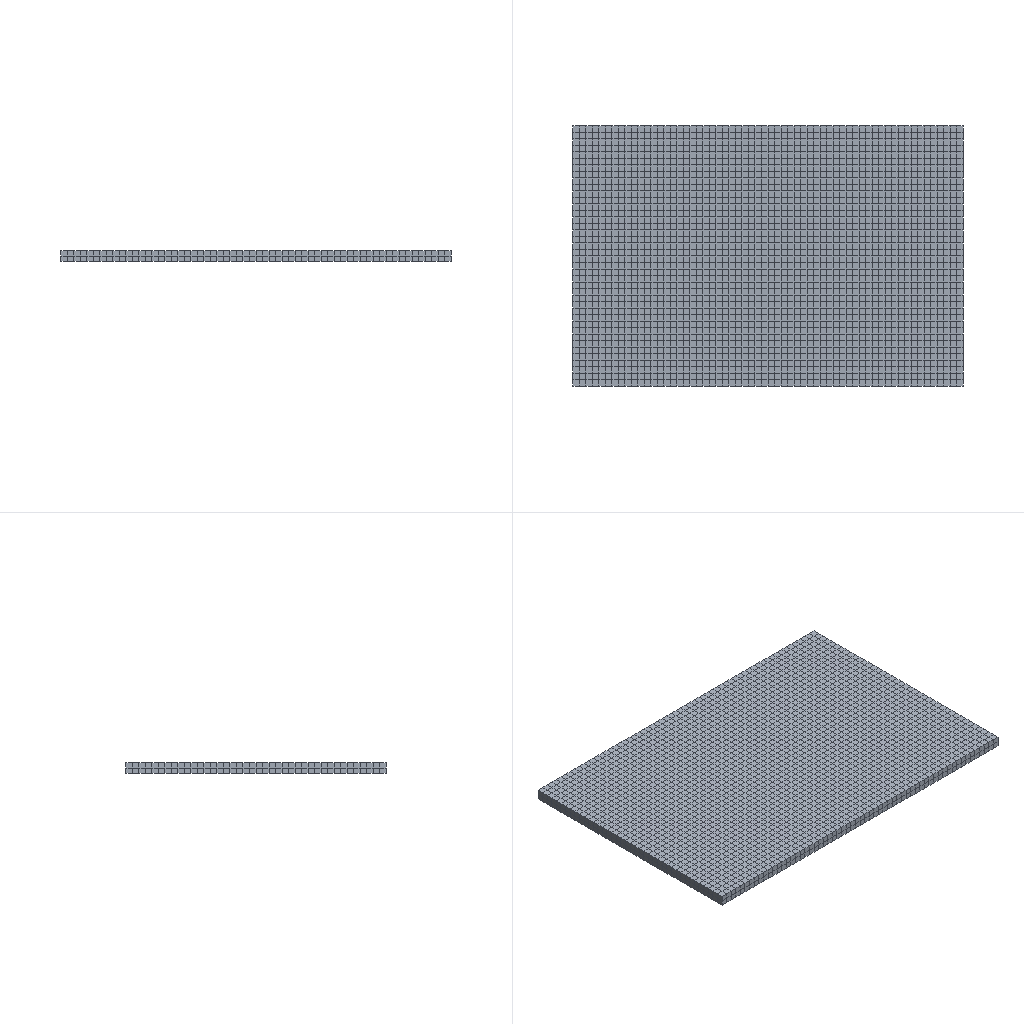Simulation study | abaqus
Set-up summary:
category,name,step,type,value,unit,region
solver,abaqus
solver,version,,,Abaqus/Standard 3DEXPERIENCE R2017x
units,not stated in the deck,,not stated
analysis,deck,,thermal,thermal
load_step,Step-1,Step-1,thermal
load_step,requested,,,1
mesh,nodes,,,7503
mesh,elements,,,4800
element_type,DC3D8,,solid,4800
load,load commands in deck,,count,3
bc,support commands in deck,,count,2
material,MATERIAL-1,,in results
check,setup vs results,,match,"per instance, exact: element labels, types and connectivity; labels of the nodes the elements use; coordinates of those nodes at SINGLE_PRECISION in 1 of 1 instance(s)"
Abaqus input file, long lists of numbers shortened:
*Heading
** Job name: Job-1 Model name: Model-1
** Generated by: Abaqus/CAE 2017
*Preprint, echo=NO, model=NO, history=NO, contact=NO
**
** PARTS
**
*Part, name=Part-1
*Node
      1,           0.,          -6.,           0.
      2,           0.,          -6.,          0.5
** (7501 more lines like these left out)
*Element, type=DC3D8
   1,  210, 2805, 5262,  563,    1,   13,  525,   52
   2, 2805,  270, 1684, 5262,   13,    2,   14,  525
** (4798 more lines like these left out)
*Nset, nset=Set-1, generate
    1,  7503,     1
*Elset, elset=Set-1, generate
    1,  4800,     1
** Section: Section-1
*Solid Section, elset=Set-1, material=Material-1
,
*End Part
**
**
** ASSEMBLY
**
*Assembly, name=Assembly
**
*Instance, name=Part-1-1, part=Part-1
          0.,           6.,           0.
*End Instance
**
*Nset, nset=Set-1, instance=Part-1-1, generate
    1,  7503,     1
*Elset, elset=Set-1, instance=Part-1-1, generate
    1,  4800,     1
*Nset, nset=Set-2, instance=Part-1-1, generate
    1,  7503,     1
*Elset, elset=Set-2, instance=Part-1-1, generate
    1,  4800,     1
*Elset, elset=_Surf-1_S6, internal, instance=Part-1-1, generate
    1,  4799,     2
*Elset, elset=_Surf-1_S1, internal, instance=Part-1-1
 2361, 2362, 2363, 2364, 2365, 2366, 2367, 2368, 2369, 2370, 2371, 2372, 2373, 2374, 2375, 2376
 2377, 2378, 2379, 2380, 2381, 2382, 2383, 2384, 2385, 2386, 2387, 2388, 2389, 2390, 2391, 2392
** (3 more lines like these left out)
*Elset, elset=_Surf-1_S2, internal, instance=Part-1-1
    1,    2,    3,    4,    5,    6,    7,    8,    9,   10,   11,   12,   13,   14,   15,   16
   17,   18,   19,   20,   21,   22,   23,   24,   25,   26,   27,   28,   29,   30,   31,   32
** (3 more lines like these left out)
*Elset, elset=_Surf-1_S5, internal, instance=Part-1-1
   39,   40,   79,   80,  119,  120,  159,  160,  199,  200,  239,  240,  279,  280,  319,  320
  359,  360,  399,  400,  439,  440,  479,  480,  519,  520,  559,  560,  599,  600,  639,  640
** (13 more lines like these left out)
*Elset, elset=_Surf-1_S4, internal, instance=Part-1-1, generate
    2,  4800,     2
*Surface, type=ELEMENT, name=Surf-1
_Surf-1_S6, S6
_Surf-1_S1, S1
_Surf-1_S2, S2
_Surf-1_S4, S4
_Surf-1_S5, S5
*Elset, elset=_Surf-2_S6, internal, instance=Part-1-1, generate
    1,  4799,     2
*Elset, elset=_Surf-2_S1, internal, instance=Part-1-1
 2361, 2362, 2363, 2364, 2365, 2366, 2367, 2368, 2369, 2370, 2371, 2372, 2373, 2374, 2375, 2376
 2377, 2378, 2379, 2380, 2381, 2382, 2383, 2384, 2385, 2386, 2387, 2388, 2389, 2390, 2391, 2392
** (3 more lines like these left out)
*Elset, elset=_Surf-2_S2, internal, instance=Part-1-1
    1,    2,    3,    4,    5,    6,    7,    8,    9,   10,   11,   12,   13,   14,   15,   16
   17,   18,   19,   20,   21,   22,   23,   24,   25,   26,   27,   28,   29,   30,   31,   32
** (3 more lines like these left out)
*Elset, elset=_Surf-2_S5, internal, instance=Part-1-1
   39,   40,   79,   80,  119,  120,  159,  160,  199,  200,  239,  240,  279,  280,  319,  320
  359,  360,  399,  400,  439,  440,  479,  480,  519,  520,  559,  560,  599,  600,  639,  640
** (13 more lines like these left out)
*Elset, elset=_Surf-2_S4, internal, instance=Part-1-1, generate
    2,  4800,     2
*Surface, type=ELEMENT, name=Surf-2
_Surf-2_S6, S6
_Surf-2_S1, S1
_Surf-2_S2, S2
_Surf-2_S4, S4
_Surf-2_S5, S5
*End Assembly
**
** MATERIALS
**
*Material, name=Material-1
*Conductivity
225.,
*Density
 2.7e-09,
*Elastic
320000., 0.25
*Expansion
 6.7e-06,
*Specific Heat
 7.8e+08,
**
** PHYSICAL CONSTANTS
**
*Physical Constants, absolute zero=-273., stefan boltzmann=5.67e-08
**
** PREDEFINED FIELDS
**
** Name: Predefined Field-1   Type: Temperature
*Initial Conditions, type=TEMPERATURE
Set-2, 20.
** ----------------------------------------------------------------
**
** STEP: Step-1
**
*Step, name=Step-1, nlgeom=NO, inc=1000
*Heat Transfer, end=PERIOD
0.1, 9., , ,
**
** LOADS
**
** Name: Load-1   Type: Body heat flux
*Dflux
Set-1, BFNU, 1.
**
** INTERACTIONS
**
** Interaction: Int-1
*Sfilm
Surf-1, F, 20., 0.002
** Interaction: Int-2
*Sradiate
Surf-2, R, 20., 0.6
**
** OUTPUT REQUESTS
**
*Restart, write, frequency=0
**
** FIELD OUTPUT: F-Output-1
**
*Output, field
*Node Output
NT, RFL
*Element Output, directions=YES
HFL, TEMP
*Output, history, frequency=0
*End Step
Results summary:
result,step,,partial,increments=0 time=0.0/9.0
result,analysis,,,thermal
result,last_loadstep,,,1
result,primary field,,,NT11